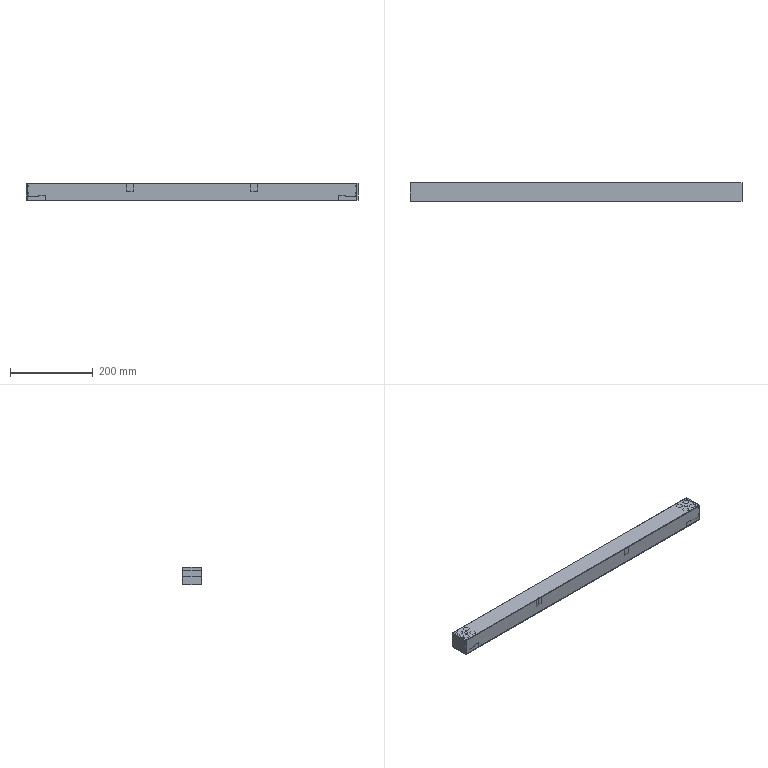NC program | NX | posted with a generic post | part box 801.8 x 45 x 42 mm
Whole program:
N10 G17 G21 G94 G90
(ZLEVEL_PROFILE_COPY_1 , TOOL : D12JING)
N12 T21 M6
N14 M5
(刀补11 , TOOL : D10JING)
N16 T11 M6
N18 G54
N20 G17 G0 G90 X401.882 Y29.743 S8000 M3
N22 G43 Z30. H11
N24 Z-5.6
N26 G94 G1 Z-6.6 F1200.
N28 G41 X401.79 Y29.705 D11
N30 X400.468 Y28.877
N32 G3 X400. Y27.994 R1.
N34 G1 X400.002 Y27.946
N36 X400.001 Y22.944
N38 X400. Y22.489
N40 Y-22.133
N42 X400.001 Y-22.58
N44 Y-27.946
N46 X400. Y-27.993
N48 G3 X400.474 Y-28.873 R1.
N50 G1 X401.793 Y-29.689
N52 G40
N54 X401.886 Y-29.726
N56 Z-5.6
N58 G0 Z30.
N60 X404.775 Y29.759
N62 Z-20.4
N64 G1 Z-21.4
N66 G41 X404.683 Y29.722
N68 X403.366 Y28.9
N70 G3 X402.897 Y28.017 R1.
N72 G1 X402.899 Y27.946
N74 X402.898 Y22.832
N76 X402.9 Y22.51
N78 Y-22.5
N80 X402.897 Y-28.017
N82 G3 X403.396 Y-28.883 R1.
N84 G1 X404.703 Y-29.639
N86 G40
N88 X404.797 Y-29.673
N90 Z-20.4
N92 G0 Z30.
N94 X-401.903 Y-29.652
N96 Z-5.6
N98 G1 Z-6.6
N100 G41 X-401.809 Y-29.618
N102 X-400.498 Y-28.861
N104 G3 X-399.998 Y-27.995 R1.
N106 G1 X-400. Y-22.133
N108 Y22.489
N110 X-400.001 Y22.5
N112 X-399.982 Y22.928
N114 X-400.001 Y22.944
N116 Y27.946
N118 X-400. Y27.993
N120 G3 X-400.474 Y28.873 R1.
N122 G1 X-401.793 Y29.689
N124 G40
N126 X-401.886 Y29.726
N128 Z-5.6
N130 G0 Z30.
N132 X-404.774 Y-29.761
N134 Z-20.4
N136 G1 Z-21.4
N138 G41 X-404.682 Y-29.723
N140 X-403.365 Y-28.9
N142 G3 X-402.896 Y-28.017 R1.
N144 G1 X-402.898 Y-27.946
N146 Y-23.027
N148 X-402.9 Y-22.5
N150 Y22.5
N152 X-402.89 Y22.817
N154 X-402.898 Y22.832
N156 Y27.946
N158 X-402.896 Y28.017
N160 G3 X-403.365 Y28.9 R1.
N162 G1 X-404.682 Y29.723
N164 G40
N166 X-404.774 Y29.761
N168 Z-20.4
N170 G0 Z30.
N172 M5
N174 M2